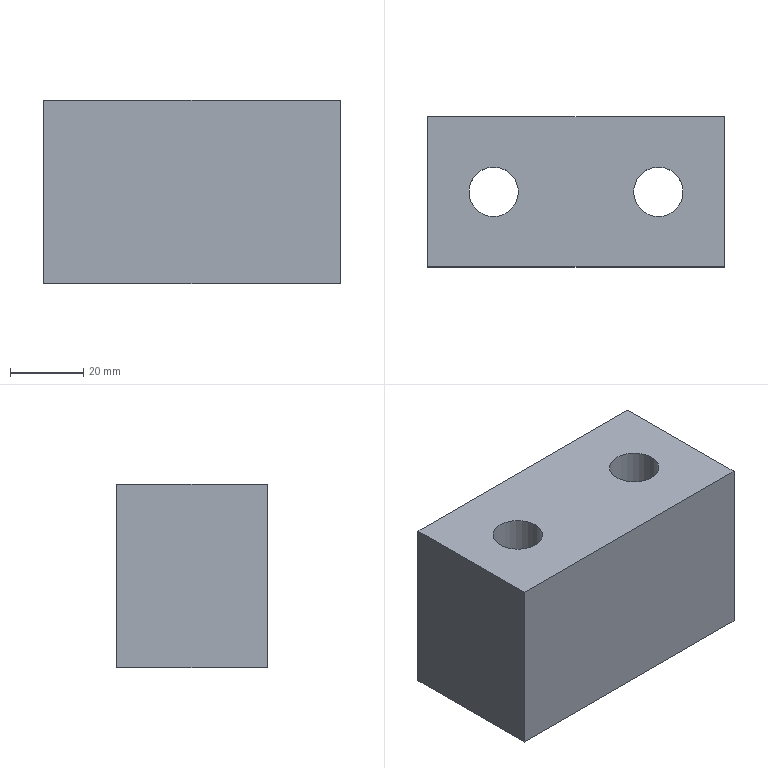Part | STEP file | lll_id754_x_t | 1 solid | 12 faces | box 81 x 41 x 50 mm | volume 142151 mm3 | plane 8 | cylinder 4 | commonest cylinder face diameters 13.509 x2 20 x2
STEP:
#1=CARTESIAN_POINT('',(974.435,57.,52.5));
#2=VERTEX_POINT('',#1);
#3=CARTESIAN_POINT('',(1055.435,57.,52.5));
#4=VERTEX_POINT('',#3);
#5=CARTESIAN_POINT('',(1017.435,57.,52.5));
#6=DIRECTION('',(1.,0.,0.));
#7=VECTOR('',#6,1.);
#8=LINE('',#5,#7);
#9=EDGE_CURVE('',#2,#4,#8,.T.);
#10=ORIENTED_EDGE('',*,*,#9,.F.);
#11=CARTESIAN_POINT('',(974.435,98.,52.5));
#12=VERTEX_POINT('',#11);
#13=CARTESIAN_POINT('',(974.435,80.,52.5));
#14=DIRECTION('',(0.,-1.,0.));
#15=VECTOR('',#14,1.);
#16=LINE('',#13,#15);
#17=EDGE_CURVE('',#12,#2,#16,.T.);
#18=ORIENTED_EDGE('',*,*,#17,.F.);
#19=CARTESIAN_POINT('',(1055.435,98.,52.5));
#20=VERTEX_POINT('',#19);
#21=CARTESIAN_POINT('',(1017.435,98.,52.5));
#22=DIRECTION('',(-1.,0.,0.));
#23=VECTOR('',#22,1.);
#24=LINE('',#21,#23);
#25=EDGE_CURVE('',#20,#12,#24,.T.);
#26=ORIENTED_EDGE('',*,*,#25,.F.);
#27=CARTESIAN_POINT('',(1055.435,80.,52.5));
#28=DIRECTION('',(0.,1.,0.));
#29=VECTOR('',#28,1.);
#30=LINE('',#27,#29);
#31=EDGE_CURVE('',#4,#20,#30,.T.);
#32=ORIENTED_EDGE('',*,*,#31,.F.);
#33=EDGE_LOOP('',(#10,#18,#26,#32));
#34=FACE_BOUND('',#33,.T.);
#35=CARTESIAN_POINT('',(1047.435,77.5,52.5));
#36=VERTEX_POINT('',#35);
#37=CARTESIAN_POINT('',(1037.435,77.5,52.5));
#38=DIRECTION('',(0.,0.,-1.));
#39=DIRECTION('',(1.,0.,0.));
#40=AXIS2_PLACEMENT_3D('',#37,#38,#39);
#41=CIRCLE('',#40,10.);
#42=EDGE_CURVE('',#36,#36,#41,.T.);
#43=ORIENTED_EDGE('',*,*,#42,.F.);
#44=EDGE_LOOP('',(#43));
#45=FACE_BOUND('',#44,.T.);
#46=CARTESIAN_POINT('',(1002.435,77.5,52.5));
#47=VERTEX_POINT('',#46);
#48=CARTESIAN_POINT('',(992.435,77.5,52.5));
#49=DIRECTION('',(0.,0.,1.));
#50=DIRECTION('',(1.,0.,0.));
#51=AXIS2_PLACEMENT_3D('',#48,#49,#50);
#52=CIRCLE('',#51,10.);
#53=EDGE_CURVE('',#47,#47,#52,.T.);
#54=ORIENTED_EDGE('',*,*,#53,.T.);
#55=EDGE_LOOP('',(#54));
#56=FACE_BOUND('',#55,.T.);
#57=CARTESIAN_POINT('',(1017.435,80.,52.5));
#58=DIRECTION('',(0.,0.,-1.));
#59=DIRECTION('',(-1.,0.,0.));
#60=AXIS2_PLACEMENT_3D('',#57,#58,#59);
#61=PLANE('',#60);
#62=ADVANCED_FACE('',(#34,#45,#56),#61,.T.);
#63=CARTESIAN_POINT('',(1055.435,57.,102.5));
#64=VERTEX_POINT('',#63);
#65=CARTESIAN_POINT('',(974.435,57.,102.5));
#66=VERTEX_POINT('',#65);
#67=CARTESIAN_POINT('',(1017.435,57.,102.5));
#68=DIRECTION('',(-1.,0.,0.));
#69=VECTOR('',#68,1.);
#70=LINE('',#67,#69);
#71=EDGE_CURVE('',#64,#66,#70,.T.);
#72=ORIENTED_EDGE('',*,*,#71,.T.);
#73=CARTESIAN_POINT('',(974.435,57.,97.5));
#74=DIRECTION('',(0.,0.,-1.));
#75=VECTOR('',#74,1.);
#76=LINE('',#73,#75);
#77=EDGE_CURVE('',#66,#2,#76,.T.);
#78=ORIENTED_EDGE('',*,*,#77,.T.);
#79=ORIENTED_EDGE('',*,*,#9,.T.);
#80=CARTESIAN_POINT('',(1055.435,57.,97.5));
#81=DIRECTION('',(0.,0.,-1.));
#82=VECTOR('',#81,1.);
#83=LINE('',#80,#82);
#84=EDGE_CURVE('',#64,#4,#83,.T.);
#85=ORIENTED_EDGE('',*,*,#84,.F.);
#86=EDGE_LOOP('',(#72,#78,#79,#85));
#87=FACE_OUTER_BOUND('',#86,.T.);
#88=CARTESIAN_POINT('',(1017.435,57.,97.5));
#89=DIRECTION('',(0.,-1.,0.));
#90=DIRECTION('',(0.,0.,1.));
#91=AXIS2_PLACEMENT_3D('',#88,#89,#90);
#92=PLANE('',#91);
#93=ADVANCED_FACE('',(#87),#92,.T.);
#94=CARTESIAN_POINT('',(1055.435,98.,102.5));
#95=VERTEX_POINT('',#94);
#96=CARTESIAN_POINT('',(1055.435,80.,102.5));
#97=DIRECTION('',(0.,1.,0.));
#98=VECTOR('',#97,1.);
#99=LINE('',#96,#98);
#100=EDGE_CURVE('',#64,#95,#99,.T.);
#101=ORIENTED_EDGE('',*,*,#100,.F.);
#102=ORIENTED_EDGE('',*,*,#84,.T.);
#103=ORIENTED_EDGE('',*,*,#31,.T.);
#104=CARTESIAN_POINT('',(1055.435,98.,97.5));
#105=DIRECTION('',(0.,0.,-1.));
#106=VECTOR('',#105,1.);
#107=LINE('',#104,#106);
#108=EDGE_CURVE('',#95,#20,#107,.T.);
#109=ORIENTED_EDGE('',*,*,#108,.F.);
#110=EDGE_LOOP('',(#101,#102,#103,#109));
#111=FACE_OUTER_BOUND('',#110,.T.);
#112=CARTESIAN_POINT('',(1055.435,80.,97.5));
#113=DIRECTION('',(1.,0.,0.));
#114=DIRECTION('',(0.,0.,-1.));
#115=AXIS2_PLACEMENT_3D('',#112,#113,#114);
#116=PLANE('',#115);
#117=ADVANCED_FACE('',(#111),#116,.T.);
#118=CARTESIAN_POINT('',(974.435,98.,102.5));
#119=VERTEX_POINT('',#118);
#120=CARTESIAN_POINT('',(1017.435,98.,102.5));
#121=DIRECTION('',(-1.,0.,0.));
#122=VECTOR('',#121,1.);
#123=LINE('',#120,#122);
#124=EDGE_CURVE('',#95,#119,#123,.T.);
#125=ORIENTED_EDGE('',*,*,#124,.F.);
#126=ORIENTED_EDGE('',*,*,#108,.T.);
#127=ORIENTED_EDGE('',*,*,#25,.T.);
#128=CARTESIAN_POINT('',(974.435,98.,97.5));
#129=DIRECTION('',(0.,0.,-1.));
#130=VECTOR('',#129,1.);
#131=LINE('',#128,#130);
#132=EDGE_CURVE('',#119,#12,#131,.T.);
#133=ORIENTED_EDGE('',*,*,#132,.F.);
#134=EDGE_LOOP('',(#125,#126,#127,#133));
#135=FACE_OUTER_BOUND('',#134,.T.);
#136=CARTESIAN_POINT('',(1017.435,98.,97.5));
#137=DIRECTION('',(0.,1.,0.));
#138=DIRECTION('',(0.,0.,-1.));
#139=AXIS2_PLACEMENT_3D('',#136,#137,#138);
#140=PLANE('',#139);
#141=ADVANCED_FACE('',(#135),#140,.T.);
#142=CARTESIAN_POINT('',(974.435,80.,102.5));
#143=DIRECTION('',(0.,1.,0.));
#144=VECTOR('',#143,1.);
#145=LINE('',#142,#144);
#146=EDGE_CURVE('',#66,#119,#145,.T.);
#147=ORIENTED_EDGE('',*,*,#146,.T.);
#148=ORIENTED_EDGE('',*,*,#132,.T.);
#149=ORIENTED_EDGE('',*,*,#17,.T.);
#150=ORIENTED_EDGE('',*,*,#77,.F.);
#151=EDGE_LOOP('',(#147,#148,#149,#150));
#152=FACE_OUTER_BOUND('',#151,.T.);
#153=CARTESIAN_POINT('',(974.435,80.,97.5));
#154=DIRECTION('',(-1.,0.,0.));
#155=DIRECTION('',(0.,0.,1.));
#156=AXIS2_PLACEMENT_3D('',#153,#154,#155);
#157=PLANE('',#156);
#158=ADVANCED_FACE('',(#152),#157,.T.);
#159=CARTESIAN_POINT('',(1027.435,77.5,80.5));
#160=VERTEX_POINT('',#159);
#161=CARTESIAN_POINT('',(1037.435,77.5,80.5));
#162=DIRECTION('',(0.,0.,1.));
#163=DIRECTION('',(-1.,0.,0.));
#164=AXIS2_PLACEMENT_3D('',#161,#162,#163);
#165=CIRCLE('',#164,10.);
#166=EDGE_CURVE('',#160,#160,#165,.T.);
#167=ORIENTED_EDGE('',*,*,#166,.T.);
#168=EDGE_LOOP('',(#167));
#169=FACE_BOUND('',#168,.T.);
#170=ORIENTED_EDGE('',*,*,#42,.T.);
#171=EDGE_LOOP('',(#170));
#172=FACE_BOUND('',#171,.T.);
#173=CARTESIAN_POINT('',(1037.435,77.5,14.3));
#174=DIRECTION('',(0.,0.,1.));
#175=DIRECTION('',(-1.,0.,0.));
#176=AXIS2_PLACEMENT_3D('',#173,#174,#175);
#177=CYLINDRICAL_SURFACE('',#176,10.);
#178=ADVANCED_FACE('',(#169,#172),#177,.F.);
#179=CARTESIAN_POINT('',(1037.435,84.255,102.5));
#180=VERTEX_POINT('',#179);
#181=CARTESIAN_POINT('',(1037.435,77.5,102.5));
#182=DIRECTION('',(0.,0.,1.));
#183=DIRECTION('',(0.,1.,0.));
#184=AXIS2_PLACEMENT_3D('',#181,#182,#183);
#185=CIRCLE('',#184,6.755);
#186=EDGE_CURVE('',#180,#180,#185,.T.);
#187=ORIENTED_EDGE('',*,*,#186,.T.);
#188=EDGE_LOOP('',(#187));
#189=FACE_BOUND('',#188,.T.);
#190=CARTESIAN_POINT('',(1037.435,70.746,80.5));
#191=VERTEX_POINT('',#190);
#192=CARTESIAN_POINT('',(1037.435,77.5,80.5));
#193=DIRECTION('',(0.,0.,1.));
#194=DIRECTION('',(0.,-1.,0.));
#195=AXIS2_PLACEMENT_3D('',#192,#193,#194);
#196=CIRCLE('',#195,6.755);
#197=EDGE_CURVE('',#191,#191,#196,.T.);
#198=ORIENTED_EDGE('',*,*,#197,.F.);
#199=EDGE_LOOP('',(#198));
#200=FACE_BOUND('',#199,.T.);
#201=CARTESIAN_POINT('',(1037.435,77.5,114.3));
#202=DIRECTION('',(0.,0.,1.));
#203=DIRECTION('',(-1.,0.,0.));
#204=AXIS2_PLACEMENT_3D('',#201,#202,#203);
#205=CYLINDRICAL_SURFACE('',#204,6.755);
#206=ADVANCED_FACE('',(#189,#200),#205,.F.);
#207=ORIENTED_EDGE('',*,*,#197,.T.);
#208=EDGE_LOOP('',(#207));
#209=FACE_BOUND('',#208,.T.);
#210=ORIENTED_EDGE('',*,*,#166,.F.);
#211=EDGE_LOOP('',(#210));
#212=FACE_BOUND('',#211,.T.);
#213=CARTESIAN_POINT('',(1037.435,77.5,80.5));
#214=DIRECTION('',(0.,0.,1.));
#215=DIRECTION('',(-1.,0.,0.));
#216=AXIS2_PLACEMENT_3D('',#213,#214,#215);
#217=PLANE('',#216);
#218=ADVANCED_FACE('',(#209,#212),#217,.F.);
#219=CARTESIAN_POINT('',(982.435,77.5,80.5));
#220=VERTEX_POINT('',#219);
#221=CARTESIAN_POINT('',(992.435,77.5,80.5));
#222=DIRECTION('',(0.,0.,-1.));
#223=DIRECTION('',(-1.,0.,0.));
#224=AXIS2_PLACEMENT_3D('',#221,#222,#223);
#225=CIRCLE('',#224,10.);
#226=EDGE_CURVE('',#220,#220,#225,.T.);
#227=ORIENTED_EDGE('',*,*,#226,.F.);
#228=EDGE_LOOP('',(#227));
#229=FACE_BOUND('',#228,.T.);
#230=ORIENTED_EDGE('',*,*,#53,.F.);
#231=EDGE_LOOP('',(#230));
#232=FACE_BOUND('',#231,.T.);
#233=CARTESIAN_POINT('',(992.435,77.5,14.3));
#234=DIRECTION('',(0.,0.,1.));
#235=DIRECTION('',(1.,0.,0.));
#236=AXIS2_PLACEMENT_3D('',#233,#234,#235);
#237=CYLINDRICAL_SURFACE('',#236,10.);
#238=ADVANCED_FACE('',(#229,#232),#237,.F.);
#239=CARTESIAN_POINT('',(992.435,84.255,102.5));
#240=VERTEX_POINT('',#239);
#241=CARTESIAN_POINT('',(992.435,77.5,102.5));
#242=DIRECTION('',(0.,0.,-1.));
#243=DIRECTION('',(0.,1.,0.));
#244=AXIS2_PLACEMENT_3D('',#241,#242,#243);
#245=CIRCLE('',#244,6.755);
#246=EDGE_CURVE('',#240,#240,#245,.T.);
#247=ORIENTED_EDGE('',*,*,#246,.F.);
#248=EDGE_LOOP('',(#247));
#249=FACE_BOUND('',#248,.T.);
#250=CARTESIAN_POINT('',(992.435,70.746,80.5));
#251=VERTEX_POINT('',#250);
#252=CARTESIAN_POINT('',(992.435,77.5,80.5));
#253=DIRECTION('',(0.,0.,-1.));
#254=DIRECTION('',(0.,-1.,0.));
#255=AXIS2_PLACEMENT_3D('',#252,#253,#254);
#256=CIRCLE('',#255,6.755);
#257=EDGE_CURVE('',#251,#251,#256,.T.);
#258=ORIENTED_EDGE('',*,*,#257,.T.);
#259=EDGE_LOOP('',(#258));
#260=FACE_BOUND('',#259,.T.);
#261=CARTESIAN_POINT('',(992.435,77.5,114.3));
#262=DIRECTION('',(0.,0.,1.));
#263=DIRECTION('',(1.,0.,0.));
#264=AXIS2_PLACEMENT_3D('',#261,#262,#263);
#265=CYLINDRICAL_SURFACE('',#264,6.755);
#266=ADVANCED_FACE('',(#249,#260),#265,.F.);
#267=ORIENTED_EDGE('',*,*,#257,.F.);
#268=EDGE_LOOP('',(#267));
#269=FACE_BOUND('',#268,.T.);
#270=ORIENTED_EDGE('',*,*,#226,.T.);
#271=EDGE_LOOP('',(#270));
#272=FACE_BOUND('',#271,.T.);
#273=CARTESIAN_POINT('',(992.435,77.5,80.5));
#274=DIRECTION('',(0.,0.,1.));
#275=DIRECTION('',(1.,0.,0.));
#276=AXIS2_PLACEMENT_3D('',#273,#274,#275);
#277=PLANE('',#276);
#278=ADVANCED_FACE('',(#269,#272),#277,.F.);
#279=ORIENTED_EDGE('',*,*,#71,.F.);
#280=ORIENTED_EDGE('',*,*,#100,.T.);
#281=ORIENTED_EDGE('',*,*,#124,.T.);
#282=ORIENTED_EDGE('',*,*,#146,.F.);
#283=EDGE_LOOP('',(#279,#280,#281,#282));
#284=FACE_BOUND('',#283,.T.);
#285=ORIENTED_EDGE('',*,*,#246,.T.);
#286=EDGE_LOOP('',(#285));
#287=FACE_BOUND('',#286,.T.);
#288=ORIENTED_EDGE('',*,*,#186,.F.);
#289=EDGE_LOOP('',(#288));
#290=FACE_BOUND('',#289,.T.);
#291=CARTESIAN_POINT('',(1134.933,-321.565,102.5));
#292=DIRECTION('',(0.,0.,-1.));
#293=DIRECTION('',(0.,1.,0.));
#294=AXIS2_PLACEMENT_3D('',#291,#292,#293);
#295=PLANE('',#294);
#296=ADVANCED_FACE('',(#284,#287,#290),#295,.F.);
#297=CLOSED_SHELL('',(#62,#93,#117,#141,#158,#178,#206,#218,#238,#266,#278,#296));
#298=MANIFOLD_SOLID_BREP('',#297);
#299=(LENGTH_UNIT()NAMED_UNIT(*)SI_UNIT(.MILLI.,.METRE.));
#300=UNCERTAINTY_MEASURE_WITH_UNIT(LENGTH_MEASURE(0.00002),#299,'','');
#301=(NAMED_UNIT(*)PLANE_ANGLE_UNIT()SI_UNIT($,.RADIAN.));
#302=PLANE_ANGLE_MEASURE_WITH_UNIT(PLANE_ANGLE_MEASURE(0.01745),#301);
#303=DIMENSIONAL_EXPONENTS(0.,0.,0.,0.,0.,0.,0.);
#304=(CONVERSION_BASED_UNIT('DEGREE',#302)NAMED_UNIT(#303)PLANE_ANGLE_UNIT());
#305=(NAMED_UNIT(*)SI_UNIT($,.STERADIAN.)SOLID_ANGLE_UNIT());
#306=(GEOMETRIC_REPRESENTATION_CONTEXT(3)GLOBAL_UNCERTAINTY_ASSIGNED_CONTEXT((#300))GLOBAL_UNIT_ASSIGNED_CONTEXT((#299,#304,#305))REPRESENTATION_CONTEXT('',''));
#307=ADVANCED_BREP_SHAPE_REPRESENTATION('',(#298),#306);